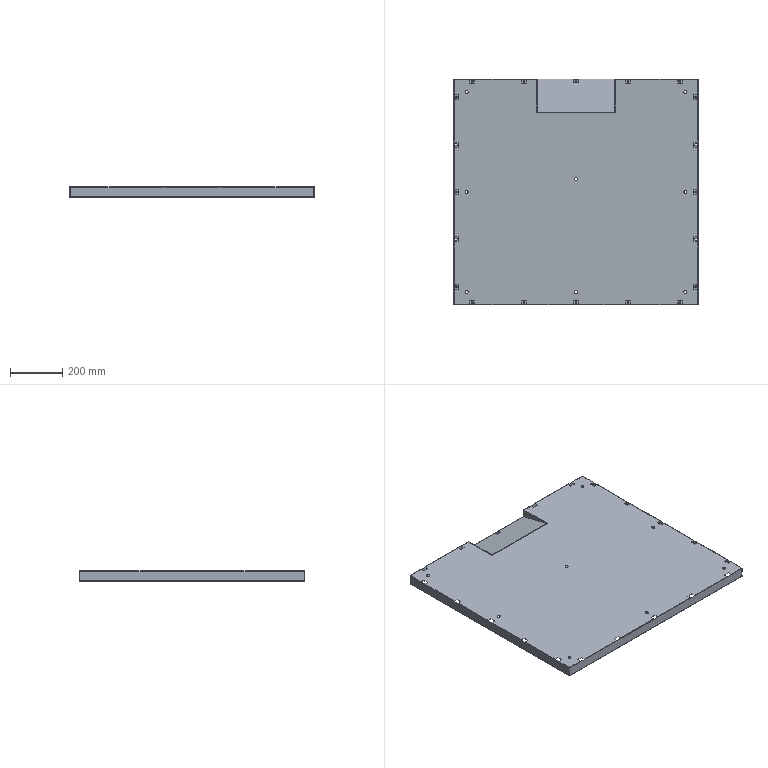Part | 2 solids | 400 faces | box 939 x 869 x 40 mm | volume 998161 mm3 | plane 254 | cylinder 126 | spline 20 | commonest cylinder face diameters 7 x50 0.4 x30 2.4 x30 11 x16